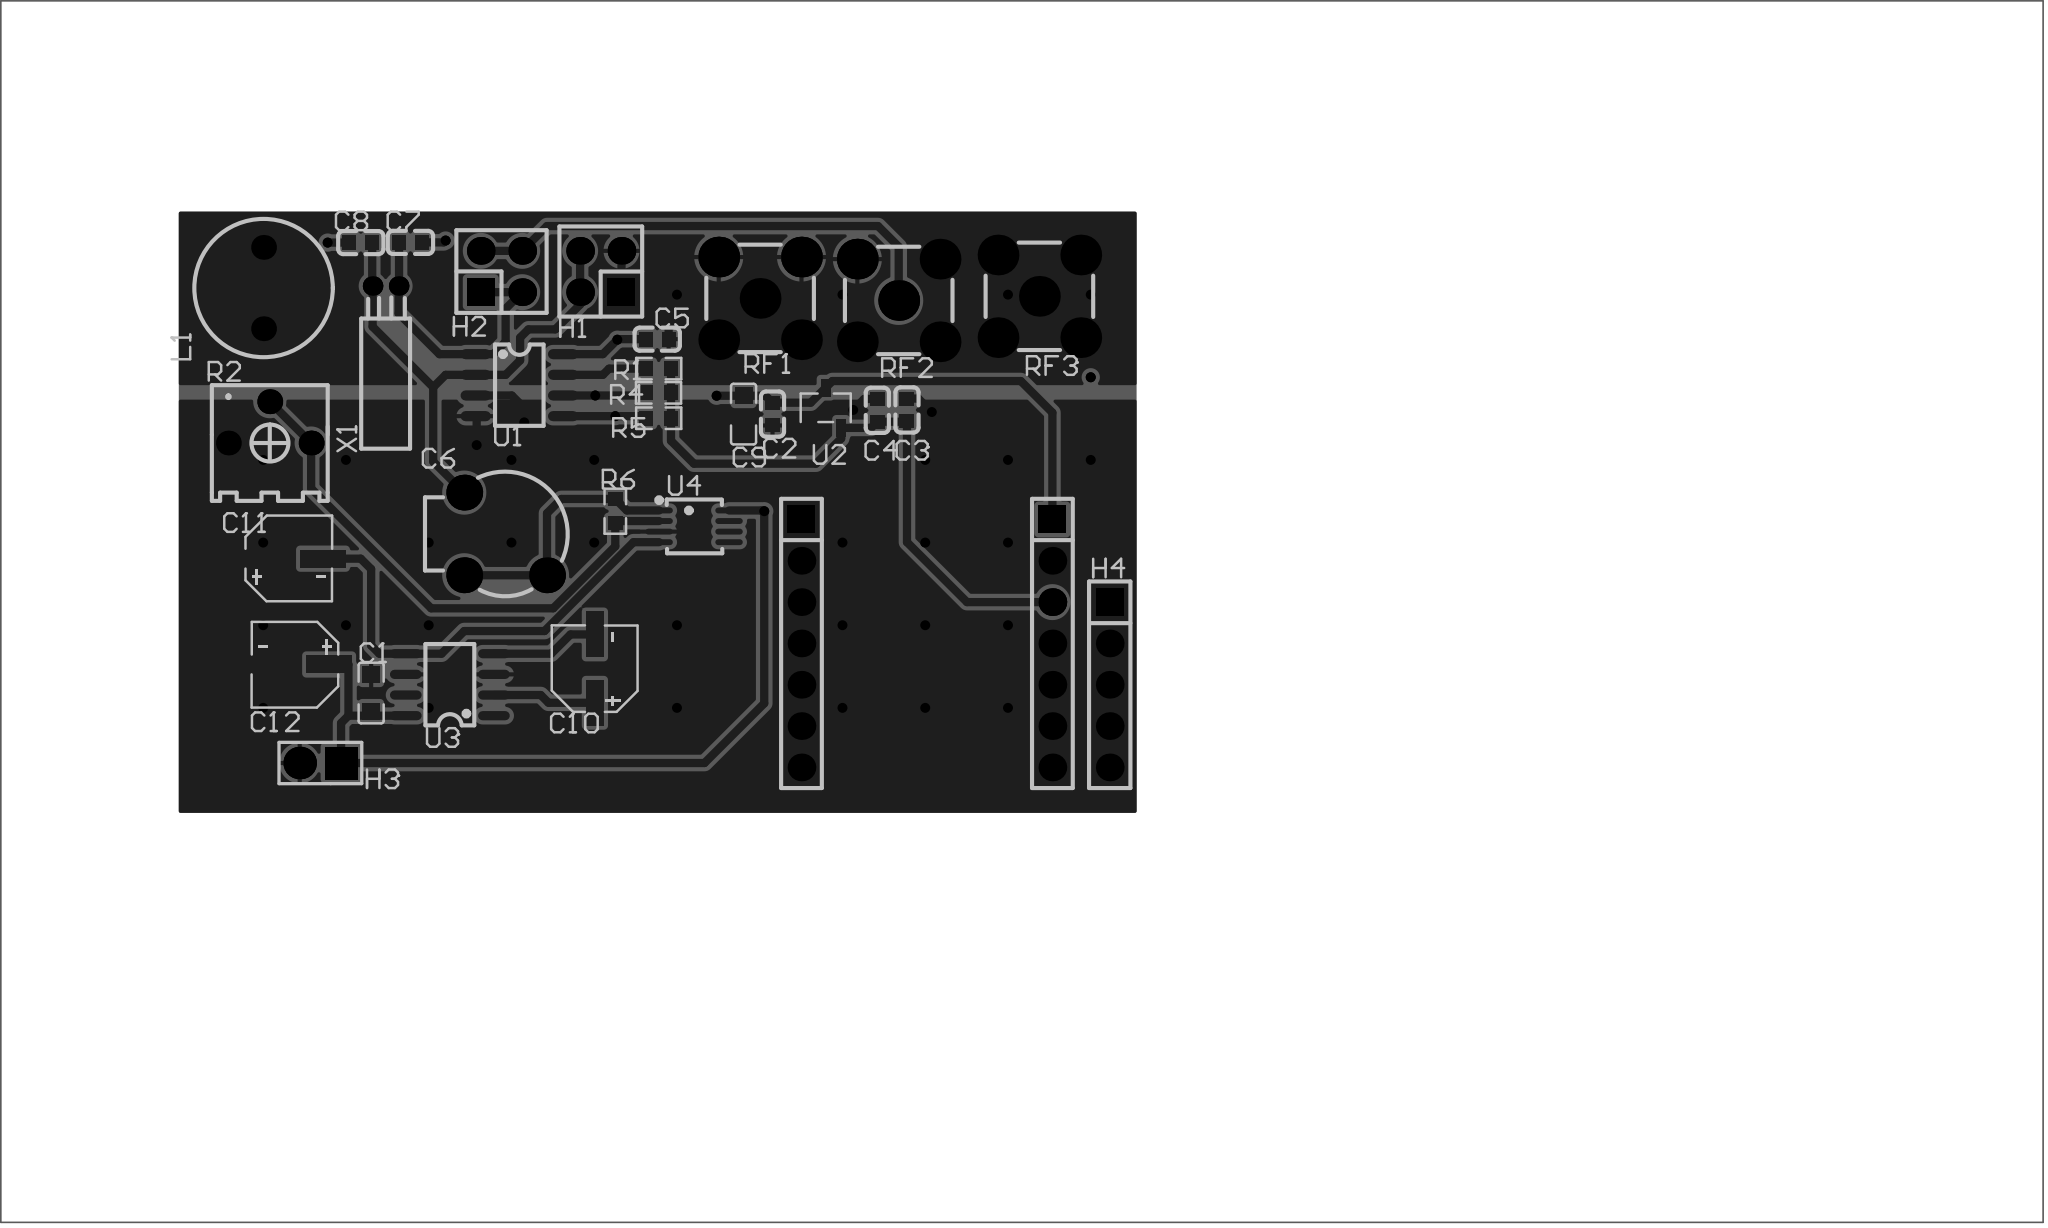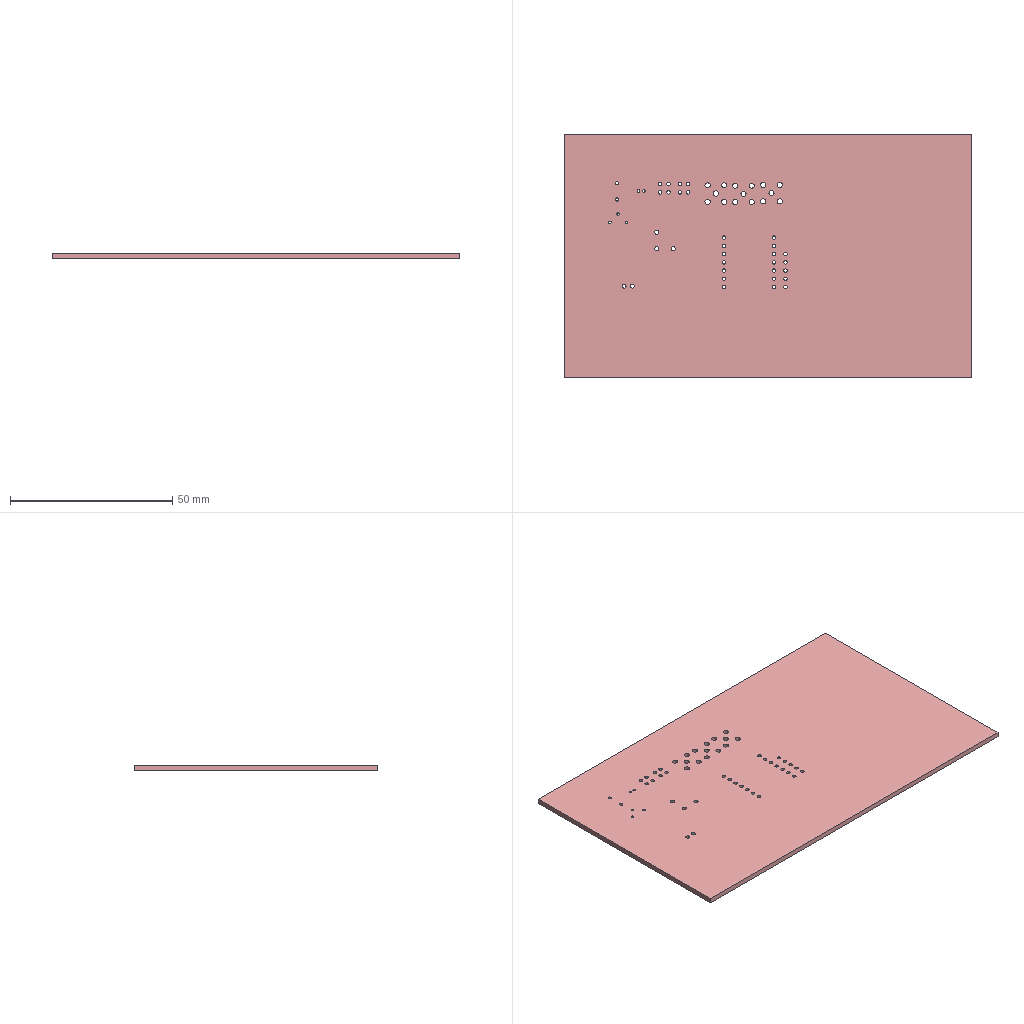Circuit board layout | Altium Designer | box 125.4 x 75.1 x 1.6 mm
Layer stack:
# Altium Designer layer stack of  (unit mm; dielectric type: 0 none, 1 core, 2 prepreg, 3 surface material)
index,name,kind,layer,copper_thickness_mm,dielectric_type,dielectric_thickness_mm,dielectric_material,dielectric_constant
0,Top Paste Mask Layer,other,,,,,,
1,Top Silkscreen Layer,other,,,,,,
2,Top Solder Mask Layer,dielectric,,,3,0.01,,3.3
3,Top Layer,copper,Top Layer,0.035,,,,
4,Dielectric1,dielectric,,,3,1.51,FR4,4.5
5,Bottom Layer,copper,Bottom Layer,0.035,,,,
6,Bottom Solder Mask Layer,dielectric,,,3,0.01,,3.3
7,Bottom Silkscreen Layer,other,,,,,,
8,Bottom Paste Mask Layer,other,,,,,,
# drill layer pairs: low layer,high layer
drill_pair,Top Layer,Bottom Layer
Part placement:
Designator,Comment,Layer,Footprint,Center-X(mm),Center-Y(mm),Rotation
C1,20uF,TopLayer,CAP-SMD_L1.8-W1.0,92.583,102.386,270
C2,100nF,TopLayer,C0603,117.221,119.531,90
C3,10uF,TopLayer,C0603,125.476,119.785,270
C4,100nF,TopLayer,C0603,123.654,119.762,270
C5,100nF,TopLayer,C0603,110.144,124.137,180
C6,3pF~33pF,TopLayer,CAP-ADJ-TH_3P-BD7.6_BFC280811339,100.838,112.165,0
C7,22pF,TopLayer,C0603,94.995,130.085,0
C8,22pF,TopLayer,C0603,91.948,130.072,180
C9,20uF,TopLayer,CAP-SMD_L1.8-W1.0,115.443,119.531,90
C10,10uF,TopLayer,CAP-SMD_BD5.0-L5.3-W5.3-LS6.0-FD,106.318,103.887,90
C11,10uF,TopLayer,CAP-SMD_BD5.0-L5.3-W5.3-LS6.0-FD,87.528,110.645,0
C12,10uF,TopLayer,CAP-SMD_BD5.0-L5.3-W5.3-LS6.0-FD,87.903,104.141,180
H1,PZ254V-12-4P,TopLayer,HDR-TH_4P-P2.54-V-M-R2-C2-S2.54,106.68,128.294,90
H2,PZ254V-12-4P,TopLayer,HDR-TH_4P-P2.54-V-M-R2-C2-S2.54,100.584,128.294,0
H3,PZ254V-11-02P,TopLayer,HDR-TH_2P-P2.54-V-M,89.467,98.084,180
H5,PZ254V-11-07P,TopLayer,HDR-TH_7P-P2.54-V-M,134.402,105.434,270
H6,PZ254V-11-07P,TopLayer,HDR-TH_7P-P2.54-V-M,118.999,105.434,270
L1,1mH,TopLayer,IND-TH_BD8.5-P5.00-D0.6,85.979,127.278,90
R1,3.3kΩ,TopLayer,R0603,110.236,122.325,0
R2,20kΩ,TopLayer,RES-ADJ-TH_3362P,86.36,119.023,0
R4,3.3kΩ,TopLayer,R0603,110.224,120.838,180
R5,3.3kΩ,TopLayer,R0603,110.236,119.277,180
R6,10kΩ,TopLayer,R0603,107.569,113.562,270
RF1,-,TopLayer,SMA-TH_KH-SMA-KE-Z,116.459,126.642,90
RF2,-,TopLayer,SMA-TH_KH-SMA-KE-Z,124.968,126.516,90
RF3,-,TopLayer,SMA-TH_KH-SMA-KE-Z,133.604,126.769,90
U1,DS1307ZN+T&R,TopLayer,SOP-8_L4.9-W3.9-P1.27-LS6.0-BL,101.685,121.309,270
U2,ME6211A33M3G-N,TopLayer,SOT-23-3_L2.9-W1.6-P1.90-LS2.8-BR,120.487,119.918,270
U3,MAX660ESA+T,TopLayer,SOIC-8_L5.0-W4.0-P1.27-LS6.0-BL,97.414,102.898,90
U4,AD8512ARMZ-REEL,TopLayer,MSOP-8_L3.0-W3.0-P0.65-LS5.0-TL,112.407,112.632,0
X1,32.768kHz,TopLayer,OSC-TH_BD3.1-P0.8-D0.3,93.472,127.405,90
H4,,TopLayer,HDR-TH_5P-P2.54-V-M,137.922,102.894,270
Pad and via stacks:
# Altium Designer via and pad stacks of  (unit mm). Each distinct definition once, with the count of objects using it.
# via: kind,start_layer,end_layer,hole_mm,diameter_mm,mode(0 simple;1 top-mid-bottom;2 full stack),diameter_per_layer,count,example_net
# pad: kind,layer,hole_mm,hole_type(0 round;1 square;2 slot),plating,top_size,top_shape(1 round;2 rect;3 octagon;9 rounded rect),mid_size,bottom_size,mode,footprint,size_per_layer,count,example
pad,Top Layer,0,0,plated,1.015x1.08,2,1.015x1.08,1.015x1.08,0,CAP-SMD_L1.8-W1.0,,4,C1.1
pad,Top Layer,0,0,plated,0.8x0.9,2,0.8x0.9,0.8x0.9,0,C0603,,12,C2.2
pad,Top Layer,0,0,plated,2.8x1.1,2,2.8x1.1,2.8x1.1,0,CAP-SMD_BD5.0-L5.3-W5.3-LS6.0-FD,,6,C10.2
pad,Top Layer,0,0,plated,0.8065x0.864,2,0.8065x0.864,0.8065x0.864,0,R0603,,8,R1.2
pad,Top Layer,0,0,plated,0.63x1.865,1,0.63x1.865,0.63x1.865,0,SOP-8_L4.9-W3.9-P1.27-LS6.0-BL,,8,U1.1
pad,Top Layer,0,0,plated,1.07x0.6,2,1.07x0.6,1.07x0.6,0,SOT-23-3_L2.9-W1.6-P1.90-LS2.8-BR,,3,U2.1
pad,Top Layer,0,0,plated,0.5684x1.95,1,0.5684x1.95,0.5684x1.95,0,SOIC-8_L5.0-W4.0-P1.27-LS6.0-BL,,8,U3.1
pad,Top Layer,0,0,plated,1.692x0.364,1,1.692x0.364,1.692x0.364,0,MSOP-8_L3.0-W3.0-P0.65-LS5.0-TL,,8,U4.5
pad,Multi-Layer,1.3,0,plated,2.2x2.2,1,2.2x2.2,2.2x2.2,0,CAP-ADJ-TH_3P-BD7.6_BFC280811339,,3,C6.1
pad,Multi-Layer,1.1,0,plated,1.7x1.7,2,1.7x1.7,1.7x1.7,0,HDR-TH_4P-P2.54-V-M-R2-C2-S2.54,,2,H1.1
pad,Multi-Layer,1.1,0,plated,1.7x1.7,1,1.7x1.7,1.7x1.7,0,HDR-TH_4P-P2.54-V-M-R2-C2-S2.54,,6,H1.2
pad,Multi-Layer,1.2,0,plated,2x2,2,2x2,2x2,0,HDR-TH_2P-P2.54-V-M,,1,H3.1
pad,Multi-Layer,1.2,0,plated,2x2,1,2x2,2x2,0,HDR-TH_2P-P2.54-V-M,,1,H3.2
pad,Multi-Layer,1.1,0,plated,1.7x1.7,2,1.7x1.7,1.7x1.7,0,HDR-TH_7P-P2.54-V-M,,2,H5.1
pad,Multi-Layer,1.1,0,plated,1.7x1.7,1,1.7x1.7,1.7x1.7,0,HDR-TH_7P-P2.54-V-M,,12,H5.2
pad,Multi-Layer,1,0,plated,1.524x1.524,1,1.524x1.524,1.524x1.524,0,IND-TH_BD8.5-P5.00-D0.6,,2,L1.1
pad,Multi-Layer,0.762,0,plated,1.524x1.524,1,1.524x1.524,1.524x1.524,0,RES-ADJ-TH_3362P,,3,R2.3
pad,Multi-Layer,1.6,0,plated,2.5x2.5,1,2.5x2.5,2.5x2.5,0,SMA-TH_KH-SMA-KE-Z,,15,RF1.5
pad,Multi-Layer,0.8,0,plated,1.2x1.2,1,1.2x1.2,1.2x1.2,0,OSC-TH_BD3.1-P0.8-D0.3,,2,X1.1
pad,Multi-Layer,1.1,0,plated,1.7x1.7,2,1.7x1.7,1.7x1.7,0,HDR-TH_5P-P2.54-V-M,,1,H4.1
pad,Multi-Layer,1.1,0,plated,1.7x1.7,1,1.7x1.7,1.7x1.7,0,HDR-TH_5P-P2.54-V-M,,4,H4.2
via,Top Layer,Bottom Layer,0.3048,0.61,0,,43,VCC
Copper pours:
name,layer,net,type(0 solid;1 hatched;2 none)
Top Layer-GND,Top Layer,GND,0
Top Layer-PGND,Top Layer,PGND,0
Bottom Layer-GND,Bottom Layer,GND,0
Design rules, without the lines most boards share:
# Altium Designer design rules of  (exported by Altium Designer, unit mm)
# columns: name | kind | enabled | priority | scope1 | scope2 | descriptor | typed fields (field=value)
copperRegion | 20 | enabled | 1 | (InNet('GND') OR InNet('PGND')) | All | Polygon Connect Rule(Relief Connect )(Conductor Width=10mil) (Relief Angle=90 Angle) (Entries=4) (Air Gap Width=10mil) ((InNet('GND') OR InNet('PGND'))),(All) | connect_style(0=relief,1=direct,2=none)=0 relief_conductor_width=0.254 relief_entries=4